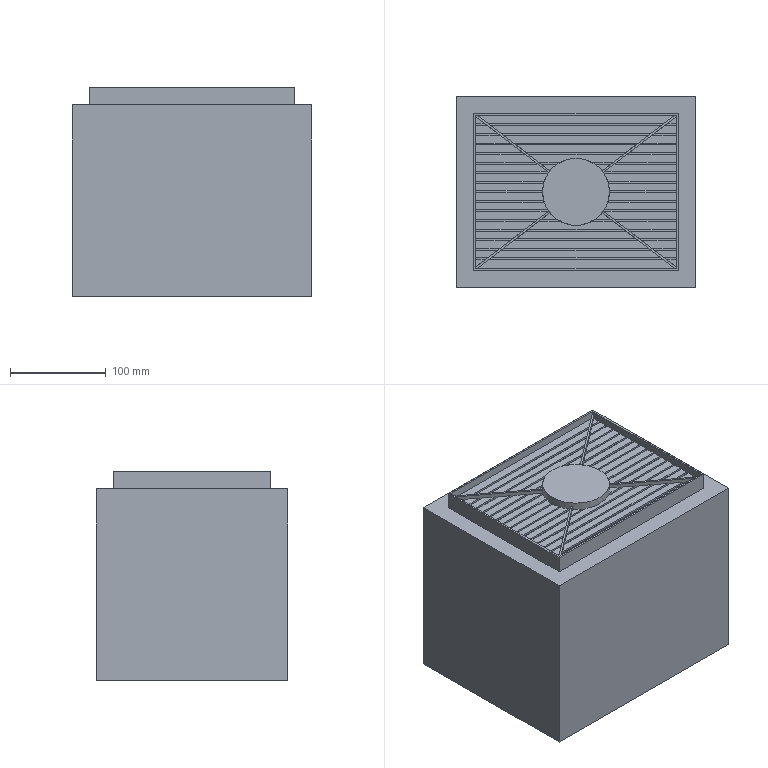Part | SolidWorks | features ICE 3, BossThin 2, Cut 2, CutThin 1, Extrusion 1, LPattern 1 | 1 solid | 210 faces | box 250 x 200 x 218 mm | volume 2929125 mm3 | plane 206 | cylinder 4 | commonest cylinder face diameters 25 x2 70 x2